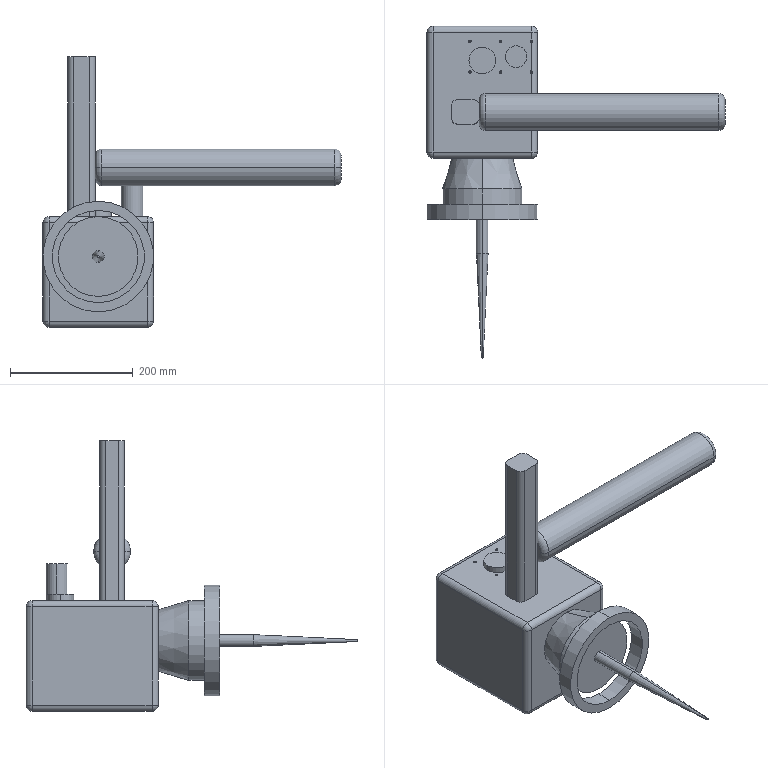Part | SolidWorks | features ICE 7, Fillet 3, Blend 1, Chamfer 1, Extrusion 1, HoleWzd 1 | 7 solids | 94 faces | box 485 x 540 x 440 mm | volume 9649241 mm3 | cylinder 42 | plane 24 | cone 16 | sphere 8 | torus 4 | commonest cylinder face diameters 20 x16 4.2 x12 19.104 x2 35 x2 43.236 x2 60 x2